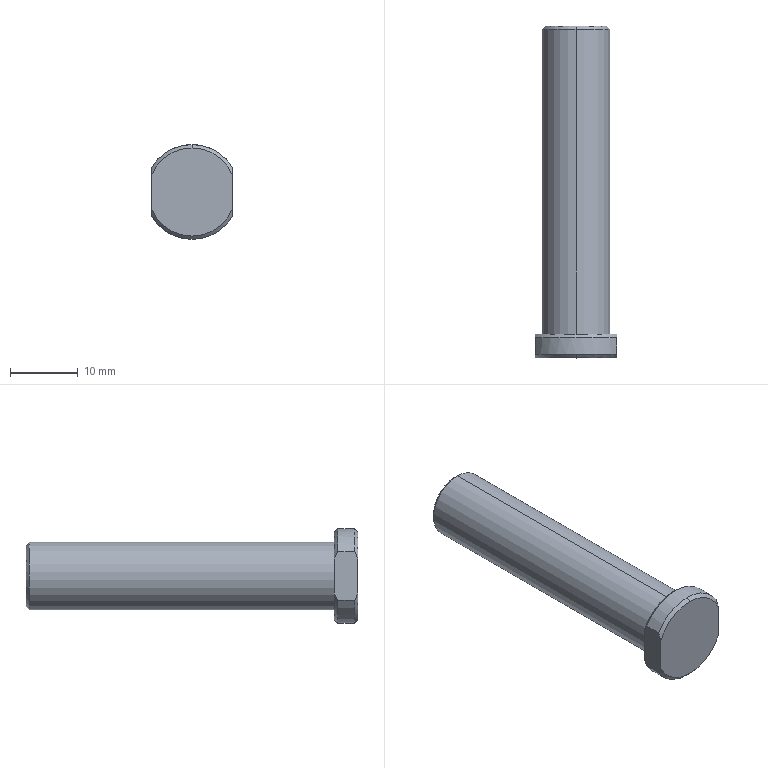Part | STEP file | (PA01.001.LX012) Idler Fixed Shaft | 1 solid | 22 faces | box 12 x 49 x 14 mm | volume 3867 mm3 | cone 10 | cylinder 7 | plane 5 | commonest cylinder face diameters 14 x3 4.2 x2 10 x2